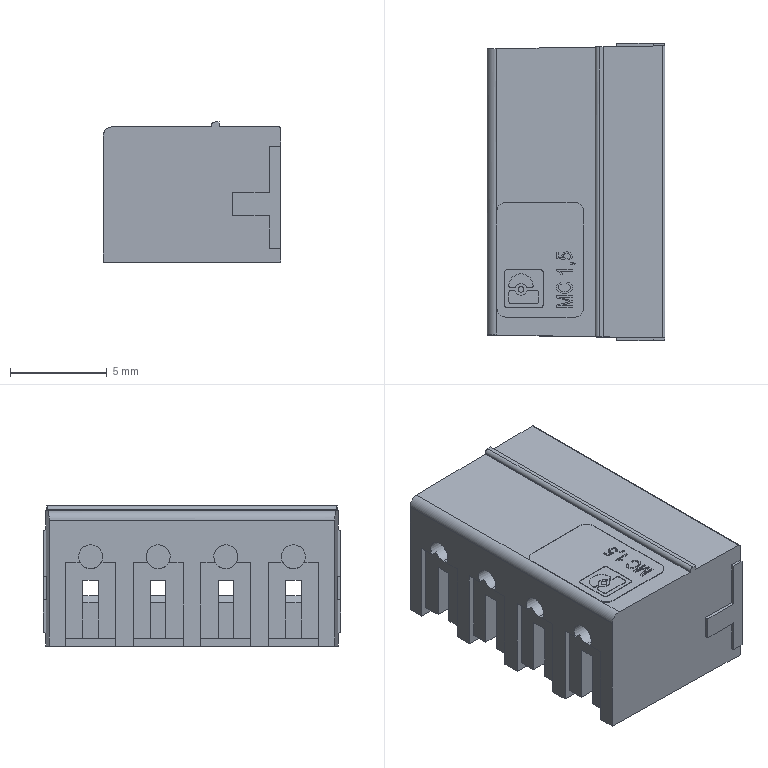Part | STEP file | RJ-USIO-V1_2-220411_289 | 1 solid | 375 faces | box 9.2 x 15.4 x 7.25 mm | volume 495.423 mm3 | plane 325 | cylinder 38 | cone 12 | commonest cylinder face diameters 0.209 x10 1.25 x8 1 x5 0.278 x4 3 x4 0.3 x2